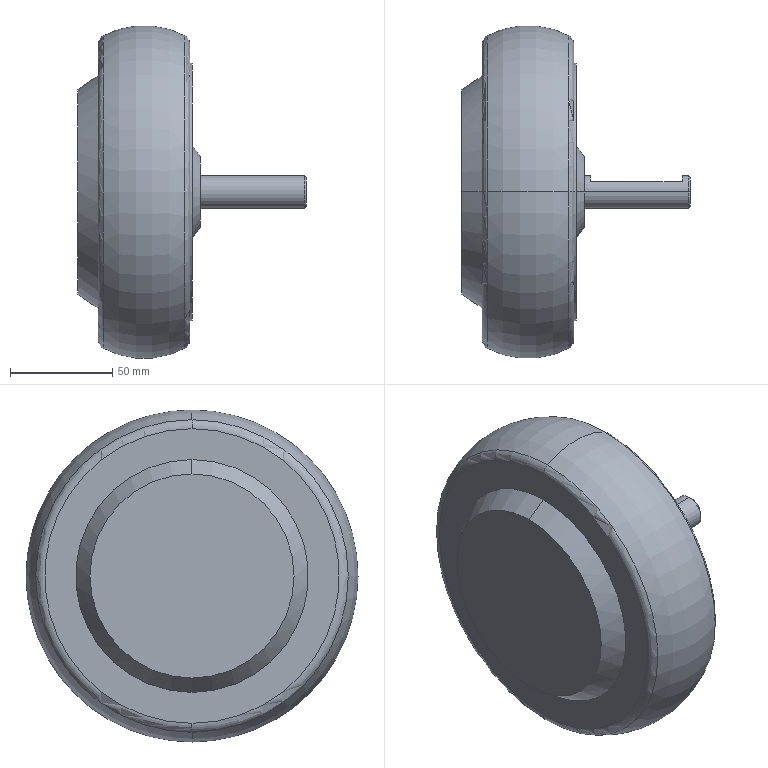Part | SolidWorks | features ICE 2, Chamfer 1, Fillet 1, Revolution 1 | 1 solid | 28 faces | box 112 x 163 x 163 mm | volume 1005033 mm3 | plane 10 | cylinder 6 | cone 6 | torus 6 | commonest cylinder face diameters 8 x2 16 x2 126 x2
STEP:
#1=CARTESIAN_POINT('',(81.577,0.,4.));
#2=VERTEX_POINT('',#1);
#3=CARTESIAN_POINT('',(81.577,0.,-4.));
#4=VERTEX_POINT('',#3);
#5=CARTESIAN_POINT('',(81.577,0.,0.));
#6=DIRECTION('',(1.,0.,0.));
#7=DIRECTION('',(0.,0.,-1.));
#8=AXIS2_PLACEMENT_3D('',#5,#6,#7);
#9=CIRCLE('',#8,4.);
#10=EDGE_CURVE('',#2,#4,#9,.T.);
#11=ORIENTED_EDGE('',*,*,#10,.F.);
#12=CARTESIAN_POINT('',(131.577,0.,4.));
#13=VERTEX_POINT('',#12);
#14=CARTESIAN_POINT('',(81.577,0.,4.));
#15=DIRECTION('',(1.,0.,0.));
#16=VECTOR('',#15,1000.);
#17=LINE('',#14,#16);
#18=EDGE_CURVE('',#2,#13,#17,.T.);
#19=ORIENTED_EDGE('',*,*,#18,.T.);
#20=CARTESIAN_POINT('',(131.577,0.,-4.));
#21=VERTEX_POINT('',#20);
#22=CARTESIAN_POINT('',(131.577,0.,0.));
#23=DIRECTION('',(1.,0.,0.));
#24=DIRECTION('',(0.,0.,-1.));
#25=AXIS2_PLACEMENT_3D('',#22,#23,#24);
#26=CIRCLE('',#25,4.);
#27=EDGE_CURVE('',#13,#21,#26,.T.);
#28=ORIENTED_EDGE('',*,*,#27,.T.);
#29=CARTESIAN_POINT('',(81.577,0.,-4.));
#30=DIRECTION('',(1.,0.,0.));
#31=VECTOR('',#30,1000.);
#32=LINE('',#29,#31);
#33=EDGE_CURVE('',#4,#21,#32,.T.);
#34=ORIENTED_EDGE('',*,*,#33,.F.);
#35=EDGE_LOOP('',(#11,#19,#28,#34));
#36=FACE_OUTER_BOUND('',#35,.T.);
#37=CARTESIAN_POINT('',(81.577,0.,0.));
#38=DIRECTION('',(1.,0.,0.));
#39=DIRECTION('',(0.,0.,-1.));
#40=AXIS2_PLACEMENT_3D('',#37,#38,#39);
#41=CYLINDRICAL_SURFACE('',#40,4.);
#42=ADVANCED_FACE('',(#36),#41,.F.);
#43=CARTESIAN_POINT('',(131.577,0.,-7.));
#44=VERTEX_POINT('',#43);
#45=CARTESIAN_POINT('',(131.577,0.,7.));
#46=VERTEX_POINT('',#45);
#47=CARTESIAN_POINT('',(131.577,0.,0.));
#48=DIRECTION('',(1.,0.,0.));
#49=DIRECTION('',(0.,0.,-1.));
#50=AXIS2_PLACEMENT_3D('',#47,#48,#49);
#51=CIRCLE('',#50,7.);
#52=EDGE_CURVE('',#44,#46,#51,.T.);
#53=ORIENTED_EDGE('',*,*,#52,.F.);
#54=CARTESIAN_POINT('',(130.577,0.,-8.));
#55=VERTEX_POINT('',#54);
#56=CARTESIAN_POINT('',(131.577,0.,-7.));
#57=DIRECTION('',(-0.7071,0.,-0.7071));
#58=VECTOR('',#57,1000.);
#59=LINE('',#56,#58);
#60=EDGE_CURVE('',#44,#55,#59,.T.);
#61=ORIENTED_EDGE('',*,*,#60,.T.);
#62=CARTESIAN_POINT('',(130.577,0.,8.));
#63=VERTEX_POINT('',#62);
#64=CARTESIAN_POINT('',(130.577,0.,0.));
#65=DIRECTION('',(-1.,0.,0.));
#66=DIRECTION('',(0.,0.,-1.));
#67=AXIS2_PLACEMENT_3D('',#64,#65,#66);
#68=CIRCLE('',#67,8.);
#69=EDGE_CURVE('',#63,#55,#68,.T.);
#70=ORIENTED_EDGE('',*,*,#69,.F.);
#71=CARTESIAN_POINT('',(131.577,0.,7.));
#72=DIRECTION('',(-0.7071,0.,0.7071));
#73=VECTOR('',#72,1000.);
#74=LINE('',#71,#73);
#75=EDGE_CURVE('',#46,#63,#74,.T.);
#76=ORIENTED_EDGE('',*,*,#75,.F.);
#77=EDGE_LOOP('',(#53,#61,#70,#76));
#78=FACE_OUTER_BOUND('',#77,.T.);
#79=CARTESIAN_POINT('',(131.577,0.,0.));
#80=DIRECTION('',(-1.,0.,0.));
#81=DIRECTION('',(0.,0.,1.));
#82=AXIS2_PLACEMENT_3D('',#79,#80,#81);
#83=CONICAL_SURFACE('',#82,7.,0.7854);
#84=ADVANCED_FACE('',(#78),#83,.T.);
#85=CARTESIAN_POINT('',(71.93,0.,76.538));
#86=VERTEX_POINT('',#85);
#87=CARTESIAN_POINT('',(71.93,0.,-76.538));
#88=VERTEX_POINT('',#87);
#89=CARTESIAN_POINT('',(71.93,0.,0.));
#90=DIRECTION('',(-1.,0.,0.));
#91=DIRECTION('',(0.,0.,1.));
#92=AXIS2_PLACEMENT_3D('',#89,#90,#91);
#93=CIRCLE('',#92,76.538);
#94=EDGE_CURVE('',#86,#88,#93,.T.);
#95=ORIENTED_EDGE('',*,*,#94,.F.);
#96=CARTESIAN_POINT('',(74.577,0.,72.126));
#97=VERTEX_POINT('',#96);
#98=CARTESIAN_POINT('',(69.577,0.,72.126));
#99=DIRECTION('',(0.,1.,0.));
#100=DIRECTION('',(0.,0.,1.));
#101=AXIS2_PLACEMENT_3D('',#98,#99,#100);
#102=CIRCLE('',#101,5.);
#103=EDGE_CURVE('',#86,#97,#102,.T.);
#104=ORIENTED_EDGE('',*,*,#103,.T.);
#105=CARTESIAN_POINT('',(74.577,0.,-72.126));
#106=VERTEX_POINT('',#105);
#107=CARTESIAN_POINT('',(74.577,0.,0.));
#108=DIRECTION('',(1.,0.,0.));
#109=DIRECTION('',(0.,0.,-1.));
#110=AXIS2_PLACEMENT_3D('',#107,#108,#109);
#111=CIRCLE('',#110,72.126);
#112=EDGE_CURVE('',#106,#97,#111,.T.);
#113=ORIENTED_EDGE('',*,*,#112,.F.);
#114=CARTESIAN_POINT('',(69.577,0.,-72.126));
#115=DIRECTION('',(0.,-1.,0.));
#116=DIRECTION('',(0.,0.,-1.));
#117=AXIS2_PLACEMENT_3D('',#114,#115,#116);
#118=CIRCLE('',#117,5.);
#119=EDGE_CURVE('',#88,#106,#118,.T.);
#120=ORIENTED_EDGE('',*,*,#119,.F.);
#121=EDGE_LOOP('',(#95,#104,#113,#120));
#122=FACE_OUTER_BOUND('',#121,.T.);
#123=CARTESIAN_POINT('',(69.577,0.,0.));
#124=DIRECTION('',(1.,0.,0.));
#125=DIRECTION('',(0.,0.,-1.));
#126=AXIS2_PLACEMENT_3D('',#123,#124,#125);
#127=TOROIDAL_SURFACE('',#126,72.126,5.);
#128=ADVANCED_FACE('',(#122),#127,.T.);
#129=CARTESIAN_POINT('',(32.225,0.,-76.538));
#130=VERTEX_POINT('',#129);
#131=CARTESIAN_POINT('',(32.225,0.,76.538));
#132=VERTEX_POINT('',#131);
#133=CARTESIAN_POINT('',(32.225,0.,0.));
#134=DIRECTION('',(1.,0.,0.));
#135=DIRECTION('',(0.,0.,-1.));
#136=AXIS2_PLACEMENT_3D('',#133,#134,#135);
#137=CIRCLE('',#136,76.538);
#138=EDGE_CURVE('',#130,#132,#137,.T.);
#139=ORIENTED_EDGE('',*,*,#138,.F.);
#140=CARTESIAN_POINT('',(29.577,0.,-72.126));
#141=VERTEX_POINT('',#140);
#142=CARTESIAN_POINT('',(34.577,0.,-72.126));
#143=DIRECTION('',(0.,1.,0.));
#144=DIRECTION('',(0.,0.,1.));
#145=AXIS2_PLACEMENT_3D('',#142,#143,#144);
#146=CIRCLE('',#145,5.);
#147=EDGE_CURVE('',#130,#141,#146,.T.);
#148=ORIENTED_EDGE('',*,*,#147,.T.);
#149=CARTESIAN_POINT('',(29.577,0.,72.126));
#150=VERTEX_POINT('',#149);
#151=CARTESIAN_POINT('',(29.577,0.,0.));
#152=DIRECTION('',(-1.,0.,0.));
#153=DIRECTION('',(0.,0.,1.));
#154=AXIS2_PLACEMENT_3D('',#151,#152,#153);
#155=CIRCLE('',#154,72.126);
#156=EDGE_CURVE('',#150,#141,#155,.T.);
#157=ORIENTED_EDGE('',*,*,#156,.F.);
#158=CARTESIAN_POINT('',(34.577,0.,72.126));
#159=DIRECTION('',(0.,-1.,0.));
#160=DIRECTION('',(0.,0.,-1.));
#161=AXIS2_PLACEMENT_3D('',#158,#159,#160);
#162=CIRCLE('',#161,5.);
#163=EDGE_CURVE('',#132,#150,#162,.T.);
#164=ORIENTED_EDGE('',*,*,#163,.F.);
#165=EDGE_LOOP('',(#139,#148,#157,#164));
#166=FACE_OUTER_BOUND('',#165,.T.);
#167=CARTESIAN_POINT('',(34.577,0.,0.));
#168=DIRECTION('',(-1.,0.,0.));
#169=DIRECTION('',(0.,0.,1.));
#170=AXIS2_PLACEMENT_3D('',#167,#168,#169);
#171=TOROIDAL_SURFACE('',#170,72.126,5.);
#172=ADVANCED_FACE('',(#166),#171,.T.);
#173=CARTESIAN_POINT('',(79.577,0.,-17.5));
#174=VERTEX_POINT('',#173);
#175=CARTESIAN_POINT('',(79.577,0.,17.5));
#176=VERTEX_POINT('',#175);
#177=CARTESIAN_POINT('',(79.577,0.,0.));
#178=DIRECTION('',(1.,0.,0.));
#179=DIRECTION('',(0.,0.,-1.));
#180=AXIS2_PLACEMENT_3D('',#177,#178,#179);
#181=CIRCLE('',#180,17.5);
#182=EDGE_CURVE('',#174,#176,#181,.T.);
#183=ORIENTED_EDGE('',*,*,#182,.F.);
#184=CARTESIAN_POINT('',(75.577,0.,-23.));
#185=VERTEX_POINT('',#184);
#186=CARTESIAN_POINT('',(79.577,0.,-17.5));
#187=DIRECTION('',(-0.5882,0.,-0.8087));
#188=VECTOR('',#187,1000.);
#189=LINE('',#186,#188);
#190=EDGE_CURVE('',#174,#185,#189,.T.);
#191=ORIENTED_EDGE('',*,*,#190,.T.);
#192=CARTESIAN_POINT('',(75.577,0.,23.));
#193=VERTEX_POINT('',#192);
#194=CARTESIAN_POINT('',(75.577,0.,0.));
#195=DIRECTION('',(1.,0.,0.));
#196=DIRECTION('',(0.,0.,-1.));
#197=AXIS2_PLACEMENT_3D('',#194,#195,#196);
#198=CIRCLE('',#197,23.);
#199=EDGE_CURVE('',#185,#193,#198,.T.);
#200=ORIENTED_EDGE('',*,*,#199,.T.);
#201=CARTESIAN_POINT('',(79.577,0.,17.5));
#202=DIRECTION('',(-0.5882,0.,0.8087));
#203=VECTOR('',#202,1000.);
#204=LINE('',#201,#203);
#205=EDGE_CURVE('',#176,#193,#204,.T.);
#206=ORIENTED_EDGE('',*,*,#205,.F.);
#207=EDGE_LOOP('',(#183,#191,#200,#206));
#208=FACE_OUTER_BOUND('',#207,.T.);
#209=CARTESIAN_POINT('',(79.577,0.,0.));
#210=DIRECTION('',(-1.,0.,0.));
#211=DIRECTION('',(0.,0.,1.));
#212=AXIS2_PLACEMENT_3D('',#209,#210,#211);
#213=CONICAL_SURFACE('',#212,17.5,0.942);
#214=ADVANCED_FACE('',(#208),#213,.T.);
#215=CARTESIAN_POINT('',(74.577,0.,-63.));
#216=VERTEX_POINT('',#215);
#217=CARTESIAN_POINT('',(74.577,0.,63.));
#218=VERTEX_POINT('',#217);
#219=CARTESIAN_POINT('',(74.577,0.,0.));
#220=DIRECTION('',(1.,0.,0.));
#221=DIRECTION('',(0.,0.,-1.));
#222=AXIS2_PLACEMENT_3D('',#219,#220,#221);
#223=CIRCLE('',#222,63.);
#224=EDGE_CURVE('',#216,#218,#223,.T.);
#225=ORIENTED_EDGE('',*,*,#224,.T.);
#226=CARTESIAN_POINT('',(75.577,0.,63.));
#227=VERTEX_POINT('',#226);
#228=CARTESIAN_POINT('',(0.,0.,63.));
#229=DIRECTION('',(1.,0.,0.));
#230=VECTOR('',#229,1000.);
#231=LINE('',#228,#230);
#232=EDGE_CURVE('',#218,#227,#231,.T.);
#233=ORIENTED_EDGE('',*,*,#232,.T.);
#234=CARTESIAN_POINT('',(75.577,0.,-63.));
#235=VERTEX_POINT('',#234);
#236=CARTESIAN_POINT('',(75.577,0.,0.));
#237=DIRECTION('',(1.,0.,0.));
#238=DIRECTION('',(0.,0.,-1.));
#239=AXIS2_PLACEMENT_3D('',#236,#237,#238);
#240=CIRCLE('',#239,63.);
#241=EDGE_CURVE('',#235,#227,#240,.T.);
#242=ORIENTED_EDGE('',*,*,#241,.F.);
#243=CARTESIAN_POINT('',(0.,0.,-63.));
#244=DIRECTION('',(1.,0.,0.));
#245=VECTOR('',#244,1000.);
#246=LINE('',#243,#245);
#247=EDGE_CURVE('',#216,#235,#246,.T.);
#248=ORIENTED_EDGE('',*,*,#247,.F.);
#249=EDGE_LOOP('',(#225,#233,#242,#248));
#250=FACE_OUTER_BOUND('',#249,.T.);
#251=CARTESIAN_POINT('',(0.,0.,0.));
#252=DIRECTION('',(1.,0.,0.));
#253=DIRECTION('',(0.,0.,-1.));
#254=AXIS2_PLACEMENT_3D('',#251,#252,#253);
#255=CYLINDRICAL_SURFACE('',#254,63.);
#256=ADVANCED_FACE('',(#250),#255,.T.);
#257=ORIENTED_EDGE('',*,*,#138,.T.);
#258=CARTESIAN_POINT('',(52.077,0.,39.308));
#259=DIRECTION('',(0.,1.,0.));
#260=DIRECTION('',(0.,0.,1.));
#261=AXIS2_PLACEMENT_3D('',#258,#259,#260);
#262=CIRCLE('',#261,42.192);
#263=EDGE_CURVE('',#132,#86,#262,.T.);
#264=ORIENTED_EDGE('',*,*,#263,.T.);
#265=ORIENTED_EDGE('',*,*,#94,.T.);
#266=CARTESIAN_POINT('',(52.077,0.,-39.308));
#267=DIRECTION('',(0.,-1.,0.));
#268=DIRECTION('',(0.,0.,-1.));
#269=AXIS2_PLACEMENT_3D('',#266,#267,#268);
#270=CIRCLE('',#269,42.192);
#271=EDGE_CURVE('',#130,#88,#270,.T.);
#272=ORIENTED_EDGE('',*,*,#271,.F.);
#273=EDGE_LOOP('',(#257,#264,#265,#272));
#274=FACE_OUTER_BOUND('',#273,.T.);
#275=CARTESIAN_POINT('',(52.077,0.,0.));
#276=DIRECTION('',(1.,0.,0.));
#277=DIRECTION('',(0.,0.,-1.));
#278=AXIS2_PLACEMENT_3D('',#275,#276,#277);
#279=TOROIDAL_SURFACE('',#278,39.308,42.192);
#280=ADVANCED_FACE('',(#274),#279,.T.);
#281=CARTESIAN_POINT('',(19.577,0.,-50.));
#282=VERTEX_POINT('',#281);
#283=CARTESIAN_POINT('',(19.577,0.,50.));
#284=VERTEX_POINT('',#283);
#285=CARTESIAN_POINT('',(19.577,0.,0.));
#286=DIRECTION('',(1.,0.,0.));
#287=DIRECTION('',(0.,0.,-1.));
#288=AXIS2_PLACEMENT_3D('',#285,#286,#287);
#289=CIRCLE('',#288,50.);
#290=EDGE_CURVE('',#282,#284,#289,.T.);
#291=ORIENTED_EDGE('',*,*,#290,.T.);
#292=CARTESIAN_POINT('',(29.577,0.,57.));
#293=VERTEX_POINT('',#292);
#294=CARTESIAN_POINT('',(29.577,0.,57.));
#295=DIRECTION('',(0.8192,0.,0.5735));
#296=VECTOR('',#295,1000.);
#297=LINE('',#294,#296);
#298=EDGE_CURVE('',#284,#293,#297,.T.);
#299=ORIENTED_EDGE('',*,*,#298,.T.);
#300=CARTESIAN_POINT('',(29.577,0.,-57.));
#301=VERTEX_POINT('',#300);
#302=CARTESIAN_POINT('',(29.577,0.,0.));
#303=DIRECTION('',(1.,0.,0.));
#304=DIRECTION('',(0.,0.,-1.));
#305=AXIS2_PLACEMENT_3D('',#302,#303,#304);
#306=CIRCLE('',#305,57.);
#307=EDGE_CURVE('',#301,#293,#306,.T.);
#308=ORIENTED_EDGE('',*,*,#307,.F.);
#309=CARTESIAN_POINT('',(29.577,0.,-57.));
#310=DIRECTION('',(0.8192,0.,-0.5735));
#311=VECTOR('',#310,1000.);
#312=LINE('',#309,#311);
#313=EDGE_CURVE('',#282,#301,#312,.T.);
#314=ORIENTED_EDGE('',*,*,#313,.F.);
#315=EDGE_LOOP('',(#291,#299,#308,#314));
#316=FACE_OUTER_BOUND('',#315,.T.);
#317=CARTESIAN_POINT('',(29.577,0.,0.));
#318=DIRECTION('',(1.,0.,0.));
#319=DIRECTION('',(0.,0.,-1.));
#320=AXIS2_PLACEMENT_3D('',#317,#318,#319);
#321=CONICAL_SURFACE('',#320,57.,0.6107);
#322=ADVANCED_FACE('',(#316),#321,.T.);
#323=CARTESIAN_POINT('',(82.577,5.,6.245));
#324=VERTEX_POINT('',#323);
#325=CARTESIAN_POINT('',(127.577,5.,6.245));
#326=VERTEX_POINT('',#325);
#327=CARTESIAN_POINT('',(82.577,5.,6.245));
#328=DIRECTION('',(1.,0.,0.));
#329=VECTOR('',#328,1000.);
#330=LINE('',#327,#329);
#331=EDGE_CURVE('',#324,#326,#330,.T.);
#332=ORIENTED_EDGE('',*,*,#331,.F.);
#333=CARTESIAN_POINT('',(82.577,5.,-6.245));
#334=VERTEX_POINT('',#333);
#335=CARTESIAN_POINT('',(82.577,0.,0.));
#336=DIRECTION('',(1.,0.,0.));
#337=DIRECTION('',(0.,0.,-1.));
#338=AXIS2_PLACEMENT_3D('',#335,#336,#337);
#339=CIRCLE('',#338,8.);
#340=EDGE_CURVE('',#334,#324,#339,.T.);
#341=ORIENTED_EDGE('',*,*,#340,.F.);
#342=CARTESIAN_POINT('',(127.577,5.,-6.245));
#343=VERTEX_POINT('',#342);
#344=CARTESIAN_POINT('',(82.577,5.,-6.245));
#345=DIRECTION('',(1.,0.,0.));
#346=VECTOR('',#345,1000.);
#347=LINE('',#344,#346);
#348=EDGE_CURVE('',#334,#343,#347,.T.);
#349=ORIENTED_EDGE('',*,*,#348,.T.);
#350=CARTESIAN_POINT('',(127.577,0.,0.));
#351=DIRECTION('',(1.,0.,0.));
#352=DIRECTION('',(0.,0.,-1.));
#353=AXIS2_PLACEMENT_3D('',#350,#351,#352);
#354=CIRCLE('',#353,8.);
#355=EDGE_CURVE('',#343,#326,#354,.T.);
#356=ORIENTED_EDGE('',*,*,#355,.T.);
#357=EDGE_LOOP('',(#332,#341,#349,#356));
#358=FACE_BOUND('',#357,.T.);
#359=CARTESIAN_POINT('',(79.577,0.,-8.));
#360=VERTEX_POINT('',#359);
#361=CARTESIAN_POINT('',(79.577,0.,8.));
#362=VERTEX_POINT('',#361);
#363=CARTESIAN_POINT('',(79.577,0.,0.));
#364=DIRECTION('',(1.,0.,0.));
#365=DIRECTION('',(0.,0.,-1.));
#366=AXIS2_PLACEMENT_3D('',#363,#364,#365);
#367=CIRCLE('',#366,8.);
#368=EDGE_CURVE('',#360,#362,#367,.T.);
#369=ORIENTED_EDGE('',*,*,#368,.T.);
#370=CARTESIAN_POINT('',(0.,0.,8.));
#371=DIRECTION('',(1.,0.,0.));
#372=VECTOR('',#371,1000.);
#373=LINE('',#370,#372);
#374=EDGE_CURVE('',#362,#63,#373,.T.);
#375=ORIENTED_EDGE('',*,*,#374,.T.);
#376=ORIENTED_EDGE('',*,*,#69,.T.);
#377=CARTESIAN_POINT('',(0.,0.,-8.));
#378=DIRECTION('',(1.,0.,0.));
#379=VECTOR('',#378,1000.);
#380=LINE('',#377,#379);
#381=EDGE_CURVE('',#360,#55,#380,.T.);
#382=ORIENTED_EDGE('',*,*,#381,.F.);
#383=EDGE_LOOP('',(#369,#375,#376,#382));
#384=FACE_OUTER_BOUND('',#383,.T.);
#385=CARTESIAN_POINT('',(0.,0.,0.));
#386=DIRECTION('',(1.,0.,0.));
#387=DIRECTION('',(0.,0.,-1.));
#388=AXIS2_PLACEMENT_3D('',#385,#386,#387);
#389=CYLINDRICAL_SURFACE('',#388,8.);
#390=ADVANCED_FACE('',(#358,#384),#389,.T.);
#391=ORIENTED_EDGE('',*,*,#374,.F.);
#392=CARTESIAN_POINT('',(79.577,0.,0.));
#393=DIRECTION('',(1.,0.,0.));
#394=DIRECTION('',(0.,0.,-1.));
#395=AXIS2_PLACEMENT_3D('',#392,#393,#394);
#396=CIRCLE('',#395,8.);
#397=EDGE_CURVE('',#362,#360,#396,.T.);
#398=ORIENTED_EDGE('',*,*,#397,.T.);
#399=ORIENTED_EDGE('',*,*,#381,.T.);
#400=CARTESIAN_POINT('',(130.577,0.,0.));
#401=DIRECTION('',(-1.,0.,0.));
#402=DIRECTION('',(0.,0.,-1.));
#403=AXIS2_PLACEMENT_3D('',#400,#401,#402);
#404=CIRCLE('',#403,8.);
#405=EDGE_CURVE('',#55,#63,#404,.T.);
#406=ORIENTED_EDGE('',*,*,#405,.T.);
#407=EDGE_LOOP('',(#391,#398,#399,#406));
#408=FACE_OUTER_BOUND('',#407,.T.);
#409=CARTESIAN_POINT('',(0.,0.,0.));
#410=DIRECTION('',(1.,0.,0.));
#411=DIRECTION('',(0.,0.,-1.));
#412=AXIS2_PLACEMENT_3D('',#409,#410,#411);
#413=CYLINDRICAL_SURFACE('',#412,8.);
#414=ADVANCED_FACE('',(#408),#413,.T.);
#415=ORIENTED_EDGE('',*,*,#298,.F.);
#416=CARTESIAN_POINT('',(19.577,0.,0.));
#417=DIRECTION('',(1.,0.,0.));
#418=DIRECTION('',(0.,0.,-1.));
#419=AXIS2_PLACEMENT_3D('',#416,#417,#418);
#420=CIRCLE('',#419,50.);
#421=EDGE_CURVE('',#284,#282,#420,.T.);
#422=ORIENTED_EDGE('',*,*,#421,.T.);
#423=ORIENTED_EDGE('',*,*,#313,.T.);
#424=CARTESIAN_POINT('',(29.577,0.,0.));
#425=DIRECTION('',(1.,0.,0.));
#426=DIRECTION('',(0.,0.,-1.));
#427=AXIS2_PLACEMENT_3D('',#424,#425,#426);
#428=CIRCLE('',#427,57.);
#429=EDGE_CURVE('',#293,#301,#428,.T.);
#430=ORIENTED_EDGE('',*,*,#429,.F.);
#431=EDGE_LOOP('',(#415,#422,#423,#430));
#432=FACE_OUTER_BOUND('',#431,.T.);
#433=CARTESIAN_POINT('',(29.577,0.,0.));
#434=DIRECTION('',(1.,0.,0.));
#435=DIRECTION('',(0.,0.,-1.));
#436=AXIS2_PLACEMENT_3D('',#433,#434,#435);
#437=CONICAL_SURFACE('',#436,57.,0.6107);
#438=ADVANCED_FACE('',(#432),#437,.T.);
#439=ORIENTED_EDGE('',*,*,#156,.T.);
#440=CARTESIAN_POINT('',(29.577,0.,0.));
#441=DIRECTION('',(-1.,0.,0.));
#442=DIRECTION('',(0.,0.,1.));
#443=AXIS2_PLACEMENT_3D('',#440,#441,#442);
#444=CIRCLE('',#443,72.126);
#445=EDGE_CURVE('',#141,#150,#444,.T.);
#446=ORIENTED_EDGE('',*,*,#445,.T.);
#447=EDGE_LOOP('',(#439,#446));
#448=FACE_OUTER_BOUND('',#447,.T.);
#449=ORIENTED_EDGE('',*,*,#307,.T.);
#450=ORIENTED_EDGE('',*,*,#429,.T.);
#451=EDGE_LOOP('',(#449,#450));
#452=FACE_BOUND('',#451,.T.);
#453=CARTESIAN_POINT('',(29.577,57.,0.));
#454=DIRECTION('',(-1.,0.,0.));
#455=DIRECTION('',(0.,0.,1.));
#456=AXIS2_PLACEMENT_3D('',#453,#454,#455);
#457=PLANE('',#456);
#458=ADVANCED_FACE('',(#448,#452),#457,.T.);
#459=ORIENTED_EDGE('',*,*,#263,.F.);
#460=CARTESIAN_POINT('',(32.225,0.,0.));
#461=DIRECTION('',(1.,0.,0.));
#462=DIRECTION('',(0.,0.,-1.));
#463=AXIS2_PLACEMENT_3D('',#460,#461,#462);
#464=CIRCLE('',#463,76.538);
#465=EDGE_CURVE('',#132,#130,#464,.T.);
#466=ORIENTED_EDGE('',*,*,#465,.T.);
#467=ORIENTED_EDGE('',*,*,#271,.T.);
#468=CARTESIAN_POINT('',(71.93,0.,0.));
#469=DIRECTION('',(-1.,0.,0.));
#470=DIRECTION('',(0.,0.,1.));
#471=AXIS2_PLACEMENT_3D('',#468,#469,#470);
#472=CIRCLE('',#471,76.538);
#473=EDGE_CURVE('',#88,#86,#472,.T.);
#474=ORIENTED_EDGE('',*,*,#473,.T.);
#475=EDGE_LOOP('',(#459,#466,#467,#474));
#476=FACE_OUTER_BOUND('',#475,.T.);
#477=CARTESIAN_POINT('',(52.077,0.,0.));
#478=DIRECTION('',(1.,0.,0.));
#479=DIRECTION('',(0.,0.,-1.));
#480=AXIS2_PLACEMENT_3D('',#477,#478,#479);
#481=TOROIDAL_SURFACE('',#480,39.308,42.192);
#482=ADVANCED_FACE('',(#476),#481,.T.);
#483=ORIENTED_EDGE('',*,*,#112,.T.);
#484=CARTESIAN_POINT('',(74.577,0.,0.));
#485=DIRECTION('',(1.,0.,0.));
#486=DIRECTION('',(0.,0.,-1.));
#487=AXIS2_PLACEMENT_3D('',#484,#485,#486);
#488=CIRCLE('',#487,72.126);
#489=EDGE_CURVE('',#97,#106,#488,.T.);
#490=ORIENTED_EDGE('',*,*,#489,.T.);
#491=EDGE_LOOP('',(#483,#490));
#492=FACE_OUTER_BOUND('',#491,.T.);
#493=ORIENTED_EDGE('',*,*,#224,.F.);
#494=CARTESIAN_POINT('',(74.577,0.,0.));
#495=DIRECTION('',(1.,0.,0.));
#496=DIRECTION('',(0.,0.,-1.));
#497=AXIS2_PLACEMENT_3D('',#494,#495,#496);
#498=CIRCLE('',#497,63.);
#499=EDGE_CURVE('',#218,#216,#498,.T.);
#500=ORIENTED_EDGE('',*,*,#499,.F.);
#501=EDGE_LOOP('',(#493,#500));
#502=FACE_BOUND('',#501,.T.);
#503=CARTESIAN_POINT('',(74.577,75.,0.));
#504=DIRECTION('',(1.,0.,0.));
#505=DIRECTION('',(0.,0.,-1.));
#506=AXIS2_PLACEMENT_3D('',#503,#504,#505);
#507=PLANE('',#506);
#508=ADVANCED_FACE('',(#492,#502),#507,.T.);
#509=ORIENTED_EDGE('',*,*,#232,.F.);
#510=ORIENTED_EDGE('',*,*,#499,.T.);
#511=ORIENTED_EDGE('',*,*,#247,.T.);
#512=CARTESIAN_POINT('',(75.577,0.,0.));
#513=DIRECTION('',(1.,0.,0.));
#514=DIRECTION('',(0.,0.,-1.));
#515=AXIS2_PLACEMENT_3D('',#512,#513,#514);
#516=CIRCLE('',#515,63.);
#517=EDGE_CURVE('',#227,#235,#516,.T.);
#518=ORIENTED_EDGE('',*,*,#517,.F.);
#519=EDGE_LOOP('',(#509,#510,#511,#518));
#520=FACE_OUTER_BOUND('',#519,.T.);
#521=CARTESIAN_POINT('',(0.,0.,0.));
#522=DIRECTION('',(1.,0.,0.));
#523=DIRECTION('',(0.,0.,-1.));
#524=AXIS2_PLACEMENT_3D('',#521,#522,#523);
#525=CYLINDRICAL_SURFACE('',#524,63.);
#526=ADVANCED_FACE('',(#520),#525,.T.);
#527=ORIENTED_EDGE('',*,*,#241,.T.);
#528=ORIENTED_EDGE('',*,*,#517,.T.);
#529=EDGE_LOOP('',(#527,#528));
#530=FACE_OUTER_BOUND('',#529,.T.);
#531=CARTESIAN_POINT('',(75.577,0.,0.));
#532=DIRECTION('',(1.,0.,0.));
#533=DIRECTION('',(0.,0.,-1.));
#534=AXIS2_PLACEMENT_3D('',#531,#532,#533);
#535=CIRCLE('',#534,23.);
#536=EDGE_CURVE('',#193,#185,#535,.T.);
#537=ORIENTED_EDGE('',*,*,#536,.F.);
#538=ORIENTED_EDGE('',*,*,#199,.F.);
#539=EDGE_LOOP('',(#537,#538));
#540=FACE_BOUND('',#539,.T.);
#541=CARTESIAN_POINT('',(75.577,63.,0.));
#542=DIRECTION('',(1.,0.,0.));
#543=DIRECTION('',(0.,0.,-1.));
#544=AXIS2_PLACEMENT_3D('',#541,#542,#543);
#545=PLANE('',#544);
#546=ADVANCED_FACE('',(#530,#540),#545,.T.);
#547=ORIENTED_EDGE('',*,*,#190,.F.);
#548=CARTESIAN_POINT('',(79.577,0.,0.));
#549=DIRECTION('',(1.,0.,0.));
#550=DIRECTION('',(0.,0.,-1.));
#551=AXIS2_PLACEMENT_3D('',#548,#549,#550);
#552=CIRCLE('',#551,17.5);
#553=EDGE_CURVE('',#176,#174,#552,.T.);
#554=ORIENTED_EDGE('',*,*,#553,.F.);
#555=ORIENTED_EDGE('',*,*,#205,.T.);
#556=ORIENTED_EDGE('',*,*,#536,.T.);
#557=EDGE_LOOP('',(#547,#554,#555,#556));
#558=FACE_OUTER_BOUND('',#557,.T.);
#559=CARTESIAN_POINT('',(79.577,0.,0.));
#560=DIRECTION('',(-1.,0.,0.));
#561=DIRECTION('',(0.,0.,1.));
#562=AXIS2_PLACEMENT_3D('',#559,#560,#561);
#563=CONICAL_SURFACE('',#562,17.5,0.942);
#564=ADVANCED_FACE('',(#558),#563,.T.);
#565=ORIENTED_EDGE('',*,*,#553,.T.);
#566=ORIENTED_EDGE('',*,*,#182,.T.);
#567=EDGE_LOOP('',(#565,#566));
#568=FACE_OUTER_BOUND('',#567,.T.);
#569=ORIENTED_EDGE('',*,*,#368,.F.);
#570=ORIENTED_EDGE('',*,*,#397,.F.);
#571=EDGE_LOOP('',(#569,#570));
#572=FACE_BOUND('',#571,.T.);
#573=CARTESIAN_POINT('',(79.577,17.5,0.));
#574=DIRECTION('',(1.,0.,0.));
#575=DIRECTION('',(0.,0.,-1.));
#576=AXIS2_PLACEMENT_3D('',#573,#574,#575);
#577=PLANE('',#576);
#578=ADVANCED_FACE('',(#568,#572),#577,.T.);
#579=CARTESIAN_POINT('',(131.577,0.,0.));
#580=DIRECTION('',(1.,0.,0.));
#581=DIRECTION('',(0.,0.,-1.));
#582=AXIS2_PLACEMENT_3D('',#579,#580,#581);
#583=CIRCLE('',#582,4.);
#584=EDGE_CURVE('',#21,#13,#583,.T.);
#585=ORIENTED_EDGE('',*,*,#584,.F.);
#586=ORIENTED_EDGE('',*,*,#27,.F.);
#587=EDGE_LOOP('',(#585,#586));
#588=FACE_BOUND('',#587,.T.);
#589=CARTESIAN_POINT('',(131.577,0.,0.));
#590=DIRECTION('',(1.,0.,0.));
#591=DIRECTION('',(0.,0.,-1.));
#592=AXIS2_PLACEMENT_3D('',#589,#590,#591);
#593=CIRCLE('',#592,7.);
#594=EDGE_CURVE('',#46,#44,#593,.T.);
#595=ORIENTED_EDGE('',*,*,#594,.T.);
#596=ORIENTED_EDGE('',*,*,#52,.T.);
#597=EDGE_LOOP('',(#595,#596));
#598=FACE_OUTER_BOUND('',#597,.T.);
#599=CARTESIAN_POINT('',(131.577,8.,0.));
#600=DIRECTION('',(1.,0.,0.));
#601=DIRECTION('',(0.,0.,-1.));
#602=AXIS2_PLACEMENT_3D('',#599,#600,#601);
#603=PLANE('',#602);
#604=ADVANCED_FACE('',(#588,#598),#603,.T.);
#605=ORIENTED_EDGE('',*,*,#290,.F.);
#606=ORIENTED_EDGE('',*,*,#421,.F.);
#607=EDGE_LOOP('',(#605,#606));
#608=FACE_OUTER_BOUND('',#607,.T.);
#609=CARTESIAN_POINT('',(19.577,0.,0.));
#610=DIRECTION('',(-1.,0.,0.));
#611=DIRECTION('',(0.,0.,1.));
#612=AXIS2_PLACEMENT_3D('',#609,#610,#611);
#613=PLANE('',#612);
#614=ADVANCED_FACE('',(#608),#613,.T.);
#615=ORIENTED_EDGE('',*,*,#147,.F.);
#616=ORIENTED_EDGE('',*,*,#465,.F.);
#617=ORIENTED_EDGE('',*,*,#163,.T.);
#618=ORIENTED_EDGE('',*,*,#445,.F.);
#619=EDGE_LOOP('',(#615,#616,#617,#618));
#620=FACE_OUTER_BOUND('',#619,.T.);
#621=CARTESIAN_POINT('',(34.577,0.,0.));
#622=DIRECTION('',(-1.,0.,0.));
#623=DIRECTION('',(0.,0.,1.));
#624=AXIS2_PLACEMENT_3D('',#621,#622,#623);
#625=TOROIDAL_SURFACE('',#624,72.126,5.);
#626=ADVANCED_FACE('',(#620),#625,.T.);
#627=ORIENTED_EDGE('',*,*,#103,.F.);
#628=ORIENTED_EDGE('',*,*,#473,.F.);
#629=ORIENTED_EDGE('',*,*,#119,.T.);
#630=ORIENTED_EDGE('',*,*,#489,.F.);
#631=EDGE_LOOP('',(#627,#628,#629,#630));
#632=FACE_OUTER_BOUND('',#631,.T.);
#633=CARTESIAN_POINT('',(69.577,0.,0.));
#634=DIRECTION('',(1.,0.,0.));
#635=DIRECTION('',(0.,0.,-1.));
#636=AXIS2_PLACEMENT_3D('',#633,#634,#635);
#637=TOROIDAL_SURFACE('',#636,72.126,5.);
#638=ADVANCED_FACE('',(#632),#637,.T.);
#639=CARTESIAN_POINT('',(127.577,5.,6.245));
#640=DIRECTION('',(0.,0.,-1.));
#641=VECTOR('',#640,1000.);
#642=LINE('',#639,#641);
#643=EDGE_CURVE('',#326,#343,#642,.T.);
#644=ORIENTED_EDGE('',*,*,#643,.T.);
#645=ORIENTED_EDGE('',*,*,#348,.F.);
#646=CARTESIAN_POINT('',(82.577,5.,6.245));
#647=DIRECTION('',(0.,0.,-1.));
#648=VECTOR('',#647,1000.);
#649=LINE('',#646,#648);
#650=EDGE_CURVE('',#324,#334,#649,.T.);
#651=ORIENTED_EDGE('',*,*,#650,.F.);
#652=ORIENTED_EDGE('',*,*,#331,.T.);
#653=EDGE_LOOP('',(#644,#645,#651,#652));
#654=FACE_OUTER_BOUND('',#653,.T.);
#655=CARTESIAN_POINT('',(82.577,5.,6.245));
#656=DIRECTION('',(0.,-1.,0.));
#657=DIRECTION('',(0.,0.,-1.));
#658=AXIS2_PLACEMENT_3D('',#655,#656,#657);
#659=PLANE('',#658);
#660=ADVANCED_FACE('',(#654),#659,.F.);
#661=ORIENTED_EDGE('',*,*,#340,.T.);
#662=ORIENTED_EDGE('',*,*,#650,.T.);
#663=EDGE_LOOP('',(#661,#662));
#664=FACE_OUTER_BOUND('',#663,.T.);
#665=CARTESIAN_POINT('',(82.577,0.,0.));
#666=DIRECTION('',(1.,0.,0.));
#667=DIRECTION('',(0.,0.,-1.));
#668=AXIS2_PLACEMENT_3D('',#665,#666,#667);
#669=PLANE('',#668);
#670=ADVANCED_FACE('',(#664),#669,.T.);
#671=ORIENTED_EDGE('',*,*,#355,.F.);
#672=ORIENTED_EDGE('',*,*,#643,.F.);
#673=EDGE_LOOP('',(#671,#672));
#674=FACE_OUTER_BOUND('',#673,.T.);
#675=CARTESIAN_POINT('',(127.577,0.,0.));
#676=DIRECTION('',(1.,0.,0.));
#677=DIRECTION('',(0.,0.,-1.));
#678=AXIS2_PLACEMENT_3D('',#675,#676,#677);
#679=PLANE('',#678);
#680=ADVANCED_FACE('',(#674),#679,.F.);
#681=ORIENTED_EDGE('',*,*,#60,.F.);
#682=ORIENTED_EDGE('',*,*,#594,.F.);
#683=ORIENTED_EDGE('',*,*,#75,.T.);
#684=ORIENTED_EDGE('',*,*,#405,.F.);
#685=EDGE_LOOP('',(#681,#682,#683,#684));
#686=FACE_OUTER_BOUND('',#685,.T.);
#687=CARTESIAN_POINT('',(131.577,0.,0.));
#688=DIRECTION('',(-1.,0.,0.));
#689=DIRECTION('',(0.,0.,1.));
#690=AXIS2_PLACEMENT_3D('',#687,#688,#689);
#691=CONICAL_SURFACE('',#690,7.,0.7854);
#692=ADVANCED_FACE('',(#686),#691,.T.);
#693=ORIENTED_EDGE('',*,*,#18,.F.);
#694=CARTESIAN_POINT('',(81.577,0.,0.));
#695=DIRECTION('',(1.,0.,0.));
#696=DIRECTION('',(0.,0.,-1.));
#697=AXIS2_PLACEMENT_3D('',#694,#695,#696);
#698=CIRCLE('',#697,4.);
#699=EDGE_CURVE('',#4,#2,#698,.T.);
#700=ORIENTED_EDGE('',*,*,#699,.F.);
#701=ORIENTED_EDGE('',*,*,#33,.T.);
#702=ORIENTED_EDGE('',*,*,#584,.T.);
#703=EDGE_LOOP('',(#693,#700,#701,#702));
#704=FACE_OUTER_BOUND('',#703,.T.);
#705=CARTESIAN_POINT('',(81.577,0.,0.));
#706=DIRECTION('',(1.,0.,0.));
#707=DIRECTION('',(0.,0.,-1.));
#708=AXIS2_PLACEMENT_3D('',#705,#706,#707);
#709=CYLINDRICAL_SURFACE('',#708,4.);
#710=ADVANCED_FACE('',(#704),#709,.F.);
#711=ORIENTED_EDGE('',*,*,#699,.T.);
#712=ORIENTED_EDGE('',*,*,#10,.T.);
#713=EDGE_LOOP('',(#711,#712));
#714=FACE_OUTER_BOUND('',#713,.T.);
#715=CARTESIAN_POINT('',(81.577,0.,0.));
#716=DIRECTION('',(1.,0.,0.));
#717=DIRECTION('',(0.,0.,-1.));
#718=AXIS2_PLACEMENT_3D('',#715,#716,#717);
#719=PLANE('',#718);
#720=ADVANCED_FACE('',(#714),#719,.T.);
#721=CLOSED_SHELL('',(#42,#84,#128,#172,#214,#256,#280,#322,#390,#414,#438,#458,#482,#508,#526,#546,#564,#578,#604,#614,#626,#638,#660,#670,#680,#692,#710,#720));
#722=MANIFOLD_SOLID_BREP('',#721);
#723=CARTESIAN_POINT('',(0.,0.,0.));
#724=DIRECTION('',(0.,0.,1.));
#725=DIRECTION('',(1.,0.,0.));
#726=AXIS2_PLACEMENT_3D('',#723,#724,#725);
#727=(LENGTH_UNIT()NAMED_UNIT(*)SI_UNIT(.MILLI.,.METRE.));
#728=UNCERTAINTY_MEASURE_WITH_UNIT(LENGTH_MEASURE(0.00001),#727,'','');
#729=(NAMED_UNIT(*)PLANE_ANGLE_UNIT()SI_UNIT($,.RADIAN.));
#730=(NAMED_UNIT(*)SI_UNIT($,.STERADIAN.)SOLID_ANGLE_UNIT());
#731=(GEOMETRIC_REPRESENTATION_CONTEXT(3)GLOBAL_UNCERTAINTY_ASSIGNED_CONTEXT((#728))GLOBAL_UNIT_ASSIGNED_CONTEXT((#727,#729,#730))REPRESENTATION_CONTEXT('',''));
#732=ADVANCED_BREP_SHAPE_REPRESENTATION('',(#722,#726),#731);